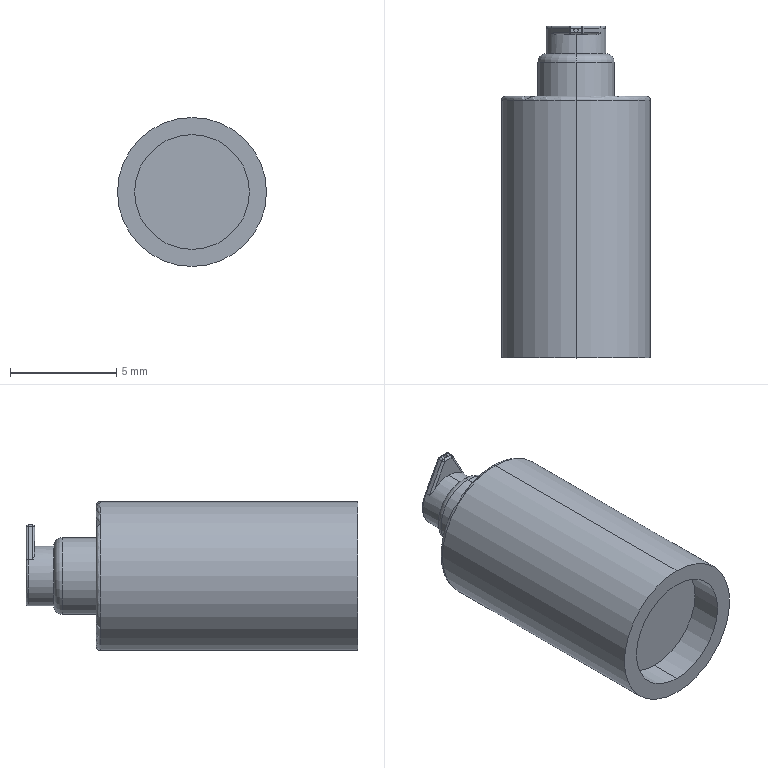Part | SolidWorks | features ICE 5, Fillet 3, Shell 2, Extrusion 1 | 1 solid | 47 faces | box 7 x 15.6 x 7 mm | volume 176.298 mm3 | cylinder 24 | plane 14 | torus 5 | sphere 4 | commonest cylinder face diameters 0.2 x10 1.8 x2 2.6 x2 2.8 x2 3.6 x2 5.4 x2
STEP:
#1=CARTESIAN_POINT('',(0.,12.1,-3.5));
#2=VERTEX_POINT('',#1);
#3=CARTESIAN_POINT('',(0.,12.1,3.5));
#4=VERTEX_POINT('',#3);
#5=CARTESIAN_POINT('',(0.,12.1,0.));
#6=DIRECTION('',(0.,-1.,0.));
#7=DIRECTION('',(0.,0.,1.));
#8=AXIS2_PLACEMENT_3D('',#5,#6,#7);
#9=CIRCLE('',#8,3.5);
#10=EDGE_CURVE('',#2,#4,#9,.T.);
#11=ORIENTED_EDGE('',*,*,#10,.F.);
#12=CARTESIAN_POINT('',(0.,12.3,-3.3));
#13=VERTEX_POINT('',#12);
#14=CARTESIAN_POINT('',(0.,12.1,-3.3));
#15=DIRECTION('',(1.,0.,0.));
#16=DIRECTION('',(0.,0.,-1.));
#17=AXIS2_PLACEMENT_3D('',#14,#15,#16);
#18=CIRCLE('',#17,0.2);
#19=EDGE_CURVE('',#2,#13,#18,.T.);
#20=ORIENTED_EDGE('',*,*,#19,.T.);
#21=CARTESIAN_POINT('',(0.,12.3,3.3));
#22=VERTEX_POINT('',#21);
#23=CARTESIAN_POINT('',(0.,12.3,0.));
#24=DIRECTION('',(0.,1.,0.));
#25=DIRECTION('',(0.,0.,1.));
#26=AXIS2_PLACEMENT_3D('',#23,#24,#25);
#27=CIRCLE('',#26,3.3);
#28=EDGE_CURVE('',#22,#13,#27,.T.);
#29=ORIENTED_EDGE('',*,*,#28,.F.);
#30=CARTESIAN_POINT('',(0.,12.1,3.3));
#31=DIRECTION('',(-1.,0.,0.));
#32=DIRECTION('',(0.,0.,1.));
#33=AXIS2_PLACEMENT_3D('',#30,#31,#32);
#34=CIRCLE('',#33,0.2);
#35=EDGE_CURVE('',#4,#22,#34,.T.);
#36=ORIENTED_EDGE('',*,*,#35,.F.);
#37=EDGE_LOOP('',(#11,#20,#29,#36));
#38=FACE_OUTER_BOUND('',#37,.T.);
#39=CARTESIAN_POINT('',(0.,12.1,0.));
#40=DIRECTION('',(0.,1.,0.));
#41=DIRECTION('',(0.,0.,1.));
#42=AXIS2_PLACEMENT_3D('',#39,#40,#41);
#43=TOROIDAL_SURFACE('',#42,3.3,0.2);
#44=ADVANCED_FACE('',(#38),#43,.T.);
#45=CARTESIAN_POINT('',(0.,13.9,-1.8));
#46=VERTEX_POINT('',#45);
#47=CARTESIAN_POINT('',(0.,13.9,1.8));
#48=VERTEX_POINT('',#47);
#49=CARTESIAN_POINT('',(0.,13.9,0.));
#50=DIRECTION('',(0.,-1.,0.));
#51=DIRECTION('',(0.,0.,1.));
#52=AXIS2_PLACEMENT_3D('',#49,#50,#51);
#53=CIRCLE('',#52,1.8);
#54=EDGE_CURVE('',#46,#48,#53,.T.);
#55=ORIENTED_EDGE('',*,*,#54,.F.);
#56=CARTESIAN_POINT('',(0.,14.3,-1.4));
#57=VERTEX_POINT('',#56);
#58=CARTESIAN_POINT('',(0.,13.9,-1.4));
#59=DIRECTION('',(1.,0.,0.));
#60=DIRECTION('',(0.,0.,-1.));
#61=AXIS2_PLACEMENT_3D('',#58,#59,#60);
#62=CIRCLE('',#61,0.4);
#63=EDGE_CURVE('',#46,#57,#62,.T.);
#64=ORIENTED_EDGE('',*,*,#63,.T.);
#65=CARTESIAN_POINT('',(0.,14.3,1.4));
#66=VERTEX_POINT('',#65);
#67=CARTESIAN_POINT('',(0.,14.3,0.));
#68=DIRECTION('',(0.,1.,0.));
#69=DIRECTION('',(0.,0.,1.));
#70=AXIS2_PLACEMENT_3D('',#67,#68,#69);
#71=CIRCLE('',#70,1.4);
#72=EDGE_CURVE('',#66,#57,#71,.T.);
#73=ORIENTED_EDGE('',*,*,#72,.F.);
#74=CARTESIAN_POINT('',(0.,13.9,1.4));
#75=DIRECTION('',(-1.,0.,0.));
#76=DIRECTION('',(0.,0.,1.));
#77=AXIS2_PLACEMENT_3D('',#74,#75,#76);
#78=CIRCLE('',#77,0.4);
#79=EDGE_CURVE('',#48,#66,#78,.T.);
#80=ORIENTED_EDGE('',*,*,#79,.F.);
#81=EDGE_LOOP('',(#55,#64,#73,#80));
#82=FACE_OUTER_BOUND('',#81,.T.);
#83=CARTESIAN_POINT('',(0.,13.9,0.));
#84=DIRECTION('',(0.,1.,0.));
#85=DIRECTION('',(0.,0.,1.));
#86=AXIS2_PLACEMENT_3D('',#83,#84,#85);
#87=TOROIDAL_SURFACE('',#86,1.4,0.4);
#88=ADVANCED_FACE('',(#82),#87,.T.);
#89=CARTESIAN_POINT('',(-0.1,15.4,2.));
#90=VERTEX_POINT('',#89);
#91=CARTESIAN_POINT('',(0.1,15.4,2.));
#92=VERTEX_POINT('',#91);
#93=CARTESIAN_POINT('',(0.,15.4,2.));
#94=DIRECTION('',(0.,0.,1.));
#95=DIRECTION('',(1.,0.,0.));
#96=AXIS2_PLACEMENT_3D('',#93,#94,#95);
#97=CIRCLE('',#96,0.1);
#98=EDGE_CURVE('',#90,#92,#97,.T.);
#99=ORIENTED_EDGE('',*,*,#98,.F.);
#100=CARTESIAN_POINT('',(-0.1,15.4,2.4));
#101=VERTEX_POINT('',#100);
#102=CARTESIAN_POINT('',(-0.1,15.4,2.));
#103=DIRECTION('',(0.,0.,1.));
#104=VECTOR('',#103,1000.);
#105=LINE('',#102,#104);
#106=EDGE_CURVE('',#90,#101,#105,.T.);
#107=ORIENTED_EDGE('',*,*,#106,.T.);
#108=CARTESIAN_POINT('',(0.,15.3,2.4));
#109=VERTEX_POINT('',#108);
#110=CARTESIAN_POINT('',(0.,15.4,2.4));
#111=DIRECTION('',(0.,0.,1.));
#112=DIRECTION('',(1.,0.,0.));
#113=AXIS2_PLACEMENT_3D('',#110,#111,#112);
#114=CIRCLE('',#113,0.1);
#115=EDGE_CURVE('',#101,#109,#114,.T.);
#116=ORIENTED_EDGE('',*,*,#115,.T.);
#117=CARTESIAN_POINT('',(0.1,15.4,2.4));
#118=VERTEX_POINT('',#117);
#119=CARTESIAN_POINT('',(0.,15.4,2.4));
#120=DIRECTION('',(0.,0.,1.));
#121=DIRECTION('',(1.,0.,0.));
#122=AXIS2_PLACEMENT_3D('',#119,#120,#121);
#123=CIRCLE('',#122,0.1);
#124=EDGE_CURVE('',#109,#118,#123,.T.);
#125=ORIENTED_EDGE('',*,*,#124,.T.);
#126=CARTESIAN_POINT('',(0.1,15.4,2.));
#127=DIRECTION('',(0.,0.,1.));
#128=VECTOR('',#127,1000.);
#129=LINE('',#126,#128);
#130=EDGE_CURVE('',#92,#118,#129,.T.);
#131=ORIENTED_EDGE('',*,*,#130,.F.);
#132=EDGE_LOOP('',(#99,#107,#116,#125,#131));
#133=FACE_OUTER_BOUND('',#132,.T.);
#134=CARTESIAN_POINT('',(0.,15.4,2.));
#135=DIRECTION('',(0.,0.,1.));
#136=DIRECTION('',(1.,0.,0.));
#137=AXIS2_PLACEMENT_3D('',#134,#135,#136);
#138=CYLINDRICAL_SURFACE('',#137,0.1);
#139=ADVANCED_FACE('',(#133),#138,.F.);
#140=CARTESIAN_POINT('',(0.,15.2,1.4));
#141=VERTEX_POINT('',#140);
#142=CARTESIAN_POINT('',(0.891,15.2,1.08));
#143=VERTEX_POINT('',#142);
#144=CARTESIAN_POINT('',(0.,15.2,0.));
#145=DIRECTION('',(0.,1.,0.));
#146=DIRECTION('',(0.,0.,1.));
#147=AXIS2_PLACEMENT_3D('',#144,#145,#146);
#148=CIRCLE('',#147,1.4);
#149=EDGE_CURVE('',#141,#143,#148,.T.);
#150=ORIENTED_EDGE('',*,*,#149,.F.);
#151=CARTESIAN_POINT('',(0.,15.6,1.4));
#152=DIRECTION('',(0.,-1.,0.));
#153=VECTOR('',#152,1000.);
#154=LINE('',#151,#153);
#155=EDGE_CURVE('',#141,#66,#154,.T.);
#156=ORIENTED_EDGE('',*,*,#155,.T.);
#157=ORIENTED_EDGE('',*,*,#72,.T.);
#158=CARTESIAN_POINT('',(0.,15.5,-1.4));
#159=VERTEX_POINT('',#158);
#160=CARTESIAN_POINT('',(0.,15.6,-1.4));
#161=DIRECTION('',(0.,-1.,0.));
#162=VECTOR('',#161,1000.);
#163=LINE('',#160,#162);
#164=EDGE_CURVE('',#159,#57,#163,.T.);
#165=ORIENTED_EDGE('',*,*,#164,.F.);
#166=CARTESIAN_POINT('',(1.171,15.5,0.7666));
#167=VERTEX_POINT('',#166);
#168=CARTESIAN_POINT('',(0.,15.5,0.));
#169=DIRECTION('',(0.,-1.,0.));
#170=DIRECTION('',(0.,0.,1.));
#171=AXIS2_PLACEMENT_3D('',#168,#169,#170);
#172=CIRCLE('',#171,1.4);
#173=EDGE_CURVE('',#159,#167,#172,.T.);
#174=ORIENTED_EDGE('',*,*,#173,.T.);
#175=CARTESIAN_POINT('',(1.171,15.3,0.7666));
#176=VERTEX_POINT('',#175);
#177=CARTESIAN_POINT('',(1.171,15.2,0.7666));
#178=DIRECTION('',(0.,1.,0.));
#179=VECTOR('',#178,1000.);
#180=LINE('',#177,#179);
#181=EDGE_CURVE('',#176,#167,#180,.T.);
#182=ORIENTED_EDGE('',*,*,#181,.F.);
#183=CARTESIAN_POINT('',(1.171,15.3,0.7666));
#184=CARTESIAN_POINT('',(1.171,15.291,0.7666));
#185=CARTESIAN_POINT('',(1.166,15.285,0.7756));
#186=CARTESIAN_POINT('',(1.156,15.277,0.7891));
#187=CARTESIAN_POINT('',(1.152,15.273,0.7961));
#188=CARTESIAN_POINT('',(1.137,15.263,0.8173));
#189=CARTESIAN_POINT('',(1.126,15.258,0.8315));
#190=CARTESIAN_POINT('',(1.095,15.242,0.8737));
#191=CARTESIAN_POINT('',(1.072,15.234,0.9012));
#192=CARTESIAN_POINT('',(1.,15.211,0.9819));
#193=CARTESIAN_POINT('',(0.9479,15.2,1.033));
#194=CARTESIAN_POINT('',(0.891,15.2,1.08));
#195=B_SPLINE_CURVE_WITH_KNOTS('',3,(#183,#184,#185,#186,#187,#188,#189,#190,#191,#192,#193,#194),.UNSPECIFIED.,.F.,.F.,(4,2,2,2,2,4),(0.,0.00002786,0.00005573,0.0001115,0.0002229,0.0004458),.UNSPECIFIED.);
#196=EDGE_CURVE('',#176,#143,#195,.T.);
#197=ORIENTED_EDGE('',*,*,#196,.T.);
#198=EDGE_LOOP('',(#150,#156,#157,#165,#174,#182,#197));
#199=FACE_OUTER_BOUND('',#198,.T.);
#200=CARTESIAN_POINT('',(0.,15.6,0.));
#201=DIRECTION('',(0.,-1.,0.));
#202=DIRECTION('',(0.,0.,-1.));
#203=AXIS2_PLACEMENT_3D('',#200,#201,#202);
#204=CYLINDRICAL_SURFACE('',#203,1.4);
#205=ADVANCED_FACE('',(#199),#204,.T.);
#206=ORIENTED_EDGE('',*,*,#54,.T.);
#207=CARTESIAN_POINT('',(0.,12.3,1.8));
#208=VERTEX_POINT('',#207);
#209=CARTESIAN_POINT('',(0.,14.3,1.8));
#210=DIRECTION('',(0.,-1.,0.));
#211=VECTOR('',#210,1000.);
#212=LINE('',#209,#211);
#213=EDGE_CURVE('',#48,#208,#212,.T.);
#214=ORIENTED_EDGE('',*,*,#213,.T.);
#215=CARTESIAN_POINT('',(0.,12.3,-1.8));
#216=VERTEX_POINT('',#215);
#217=CARTESIAN_POINT('',(0.,12.3,0.));
#218=DIRECTION('',(0.,1.,0.));
#219=DIRECTION('',(0.,0.,1.));
#220=AXIS2_PLACEMENT_3D('',#217,#218,#219);
#221=CIRCLE('',#220,1.8);
#222=EDGE_CURVE('',#208,#216,#221,.T.);
#223=ORIENTED_EDGE('',*,*,#222,.T.);
#224=CARTESIAN_POINT('',(0.,14.3,-1.8));
#225=DIRECTION('',(0.,-1.,0.));
#226=VECTOR('',#225,1000.);
#227=LINE('',#224,#226);
#228=EDGE_CURVE('',#46,#216,#227,.T.);
#229=ORIENTED_EDGE('',*,*,#228,.F.);
#230=EDGE_LOOP('',(#206,#214,#223,#229));
#231=FACE_OUTER_BOUND('',#230,.T.);
#232=CARTESIAN_POINT('',(0.,14.3,0.));
#233=DIRECTION('',(0.,-1.,0.));
#234=DIRECTION('',(0.,0.,-1.));
#235=AXIS2_PLACEMENT_3D('',#232,#233,#234);
#236=CYLINDRICAL_SURFACE('',#235,1.8);
#237=ADVANCED_FACE('',(#231),#236,.T.);
#238=CARTESIAN_POINT('',(0.,1.5,-2.7));
#239=VERTEX_POINT('',#238);
#240=CARTESIAN_POINT('',(0.,1.5,2.7));
#241=VERTEX_POINT('',#240);
#242=CARTESIAN_POINT('',(0.,1.5,0.));
#243=DIRECTION('',(0.,1.,0.));
#244=DIRECTION('',(0.,0.,1.));
#245=AXIS2_PLACEMENT_3D('',#242,#243,#244);
#246=CIRCLE('',#245,2.7);
#247=EDGE_CURVE('',#239,#241,#246,.T.);
#248=ORIENTED_EDGE('',*,*,#247,.T.);
#249=CARTESIAN_POINT('',(0.,0.,2.7));
#250=VERTEX_POINT('',#249);
#251=CARTESIAN_POINT('',(0.,2.3,2.7));
#252=DIRECTION('',(0.,-1.,0.));
#253=VECTOR('',#252,1000.);
#254=LINE('',#251,#253);
#255=EDGE_CURVE('',#241,#250,#254,.T.);
#256=ORIENTED_EDGE('',*,*,#255,.T.);
#257=CARTESIAN_POINT('',(0.,0.,-2.7));
#258=VERTEX_POINT('',#257);
#259=CARTESIAN_POINT('',(0.,0.,0.));
#260=DIRECTION('',(0.,1.,0.));
#261=DIRECTION('',(0.,0.,1.));
#262=AXIS2_PLACEMENT_3D('',#259,#260,#261);
#263=CIRCLE('',#262,2.7);
#264=EDGE_CURVE('',#258,#250,#263,.T.);
#265=ORIENTED_EDGE('',*,*,#264,.F.);
#266=CARTESIAN_POINT('',(0.,2.3,-2.7));
#267=DIRECTION('',(0.,-1.,0.));
#268=VECTOR('',#267,1000.);
#269=LINE('',#266,#268);
#270=EDGE_CURVE('',#239,#258,#269,.T.);
#271=ORIENTED_EDGE('',*,*,#270,.F.);
#272=EDGE_LOOP('',(#248,#256,#265,#271));
#273=FACE_OUTER_BOUND('',#272,.T.);
#274=CARTESIAN_POINT('',(0.,2.3,0.));
#275=DIRECTION('',(0.,-1.,0.));
#276=DIRECTION('',(0.,0.,-1.));
#277=AXIS2_PLACEMENT_3D('',#274,#275,#276);
#278=CYLINDRICAL_SURFACE('',#277,2.7);
#279=ADVANCED_FACE('',(#273),#278,.F.);
#280=ORIENTED_EDGE('',*,*,#10,.T.);
#281=CARTESIAN_POINT('',(0.,0.,3.5));
#282=VERTEX_POINT('',#281);
#283=CARTESIAN_POINT('',(0.,2.3,3.5));
#284=DIRECTION('',(0.,-1.,0.));
#285=VECTOR('',#284,1000.);
#286=LINE('',#283,#285);
#287=EDGE_CURVE('',#4,#282,#286,.T.);
#288=ORIENTED_EDGE('',*,*,#287,.T.);
#289=CARTESIAN_POINT('',(0.,0.,-3.5));
#290=VERTEX_POINT('',#289);
#291=CARTESIAN_POINT('',(0.,0.,0.));
#292=DIRECTION('',(0.,1.,0.));
#293=DIRECTION('',(0.,0.,1.));
#294=AXIS2_PLACEMENT_3D('',#291,#292,#293);
#295=CIRCLE('',#294,3.5);
#296=EDGE_CURVE('',#282,#290,#295,.T.);
#297=ORIENTED_EDGE('',*,*,#296,.T.);
#298=CARTESIAN_POINT('',(0.,2.3,-3.5));
#299=DIRECTION('',(0.,-1.,0.));
#300=VECTOR('',#299,1000.);
#301=LINE('',#298,#300);
#302=EDGE_CURVE('',#2,#290,#301,.T.);
#303=ORIENTED_EDGE('',*,*,#302,.F.);
#304=EDGE_LOOP('',(#280,#288,#297,#303));
#305=FACE_OUTER_BOUND('',#304,.T.);
#306=CARTESIAN_POINT('',(0.,2.3,0.));
#307=DIRECTION('',(0.,-1.,0.));
#308=DIRECTION('',(0.,0.,-1.));
#309=AXIS2_PLACEMENT_3D('',#306,#307,#308);
#310=CYLINDRICAL_SURFACE('',#309,3.5);
#311=ADVANCED_FACE('',(#305),#310,.T.);
#312=CARTESIAN_POINT('',(0.24,15.3,2.4));
#313=VERTEX_POINT('',#312);
#314=CARTESIAN_POINT('',(0.24,15.5,2.4));
#315=VERTEX_POINT('',#314);
#316=CARTESIAN_POINT('',(0.24,15.2,2.4));
#317=DIRECTION('',(0.,1.,0.));
#318=VECTOR('',#317,1000.);
#319=LINE('',#316,#318);
#320=EDGE_CURVE('',#313,#315,#319,.T.);
#321=ORIENTED_EDGE('',*,*,#320,.T.);
#322=CARTESIAN_POINT('',(0.,15.5,2.4));
#323=VERTEX_POINT('',#322);
#324=CARTESIAN_POINT('',(-0.3,15.5,2.4));
#325=DIRECTION('',(-1.,0.,0.));
#326=VECTOR('',#325,1000.);
#327=LINE('',#324,#326);
#328=EDGE_CURVE('',#315,#323,#327,.T.);
#329=ORIENTED_EDGE('',*,*,#328,.T.);
#330=CARTESIAN_POINT('',(0.,15.4,2.4));
#331=DIRECTION('',(0.,0.,1.));
#332=DIRECTION('',(1.,0.,0.));
#333=AXIS2_PLACEMENT_3D('',#330,#331,#332);
#334=CIRCLE('',#333,0.1);
#335=EDGE_CURVE('',#118,#323,#334,.T.);
#336=ORIENTED_EDGE('',*,*,#335,.F.);
#337=ORIENTED_EDGE('',*,*,#124,.F.);
#338=CARTESIAN_POINT('',(0.3,15.3,2.4));
#339=DIRECTION('',(1.,0.,0.));
#340=VECTOR('',#339,1000.);
#341=LINE('',#338,#340);
#342=EDGE_CURVE('',#109,#313,#341,.T.);
#343=ORIENTED_EDGE('',*,*,#342,.T.);
#344=EDGE_LOOP('',(#321,#329,#336,#337,#343));
#345=FACE_OUTER_BOUND('',#344,.T.);
#346=CARTESIAN_POINT('',(-0.3,15.2,2.4));
#347=DIRECTION('',(0.,0.,1.));
#348=DIRECTION('',(1.,0.,0.));
#349=AXIS2_PLACEMENT_3D('',#346,#347,#348);
#350=PLANE('',#349);
#351=ADVANCED_FACE('',(#345),#350,.T.);
#352=ORIENTED_EDGE('',*,*,#287,.F.);
#353=CARTESIAN_POINT('',(0.,12.1,0.));
#354=DIRECTION('',(0.,-1.,0.));
#355=DIRECTION('',(0.,0.,1.));
#356=AXIS2_PLACEMENT_3D('',#353,#354,#355);
#357=CIRCLE('',#356,3.5);
#358=EDGE_CURVE('',#4,#2,#357,.T.);
#359=ORIENTED_EDGE('',*,*,#358,.T.);
#360=ORIENTED_EDGE('',*,*,#302,.T.);
#361=CARTESIAN_POINT('',(0.,0.,0.));
#362=DIRECTION('',(0.,1.,0.));
#363=DIRECTION('',(0.,0.,1.));
#364=AXIS2_PLACEMENT_3D('',#361,#362,#363);
#365=CIRCLE('',#364,3.5);
#366=EDGE_CURVE('',#290,#282,#365,.T.);
#367=ORIENTED_EDGE('',*,*,#366,.T.);
#368=EDGE_LOOP('',(#352,#359,#360,#367));
#369=FACE_OUTER_BOUND('',#368,.T.);
#370=CARTESIAN_POINT('',(0.,2.3,0.));
#371=DIRECTION('',(0.,-1.,0.));
#372=DIRECTION('',(0.,0.,-1.));
#373=AXIS2_PLACEMENT_3D('',#370,#371,#372);
#374=CYLINDRICAL_SURFACE('',#373,3.5);
#375=ADVANCED_FACE('',(#369),#374,.T.);
#376=ORIENTED_EDGE('',*,*,#264,.T.);
#377=CARTESIAN_POINT('',(0.,0.,0.));
#378=DIRECTION('',(0.,1.,0.));
#379=DIRECTION('',(0.,0.,1.));
#380=AXIS2_PLACEMENT_3D('',#377,#378,#379);
#381=CIRCLE('',#380,2.7);
#382=EDGE_CURVE('',#250,#258,#381,.T.);
#383=ORIENTED_EDGE('',*,*,#382,.T.);
#384=EDGE_LOOP('',(#376,#383));
#385=FACE_BOUND('',#384,.T.);
#386=ORIENTED_EDGE('',*,*,#366,.F.);
#387=ORIENTED_EDGE('',*,*,#296,.F.);
#388=EDGE_LOOP('',(#386,#387));
#389=FACE_OUTER_BOUND('',#388,.T.);
#390=CARTESIAN_POINT('',(0.,0.,0.));
#391=DIRECTION('',(0.,1.,0.));
#392=DIRECTION('',(0.,0.,1.));
#393=AXIS2_PLACEMENT_3D('',#390,#391,#392);
#394=PLANE('',#393);
#395=ADVANCED_FACE('',(#385,#389),#394,.F.);
#396=ORIENTED_EDGE('',*,*,#255,.F.);
#397=CARTESIAN_POINT('',(0.,1.5,0.));
#398=DIRECTION('',(0.,1.,0.));
#399=DIRECTION('',(0.,0.,1.));
#400=AXIS2_PLACEMENT_3D('',#397,#398,#399);
#401=CIRCLE('',#400,2.7);
#402=EDGE_CURVE('',#241,#239,#401,.T.);
#403=ORIENTED_EDGE('',*,*,#402,.T.);
#404=ORIENTED_EDGE('',*,*,#270,.T.);
#405=ORIENTED_EDGE('',*,*,#382,.F.);
#406=EDGE_LOOP('',(#396,#403,#404,#405));
#407=FACE_OUTER_BOUND('',#406,.T.);
#408=CARTESIAN_POINT('',(0.,2.3,0.));
#409=DIRECTION('',(0.,-1.,0.));
#410=DIRECTION('',(0.,0.,-1.));
#411=AXIS2_PLACEMENT_3D('',#408,#409,#410);
#412=CYLINDRICAL_SURFACE('',#411,2.7);
#413=ADVANCED_FACE('',(#407),#412,.F.);
#414=ORIENTED_EDGE('',*,*,#247,.F.);
#415=ORIENTED_EDGE('',*,*,#402,.F.);
#416=EDGE_LOOP('',(#414,#415));
#417=FACE_OUTER_BOUND('',#416,.T.);
#418=CARTESIAN_POINT('',(0.,1.5,0.));
#419=DIRECTION('',(0.,1.,0.));
#420=DIRECTION('',(0.,0.,1.));
#421=AXIS2_PLACEMENT_3D('',#418,#419,#420);
#422=PLANE('',#421);
#423=ADVANCED_FACE('',(#417),#422,.F.);
#424=ORIENTED_EDGE('',*,*,#28,.T.);
#425=CARTESIAN_POINT('',(0.,12.3,0.));
#426=DIRECTION('',(0.,1.,0.));
#427=DIRECTION('',(0.,0.,1.));
#428=AXIS2_PLACEMENT_3D('',#425,#426,#427);
#429=CIRCLE('',#428,3.3);
#430=EDGE_CURVE('',#13,#22,#429,.T.);
#431=ORIENTED_EDGE('',*,*,#430,.T.);
#432=EDGE_LOOP('',(#424,#431));
#433=FACE_OUTER_BOUND('',#432,.T.);
#434=CARTESIAN_POINT('',(0.,12.3,0.));
#435=DIRECTION('',(0.,1.,0.));
#436=DIRECTION('',(0.,0.,1.));
#437=AXIS2_PLACEMENT_3D('',#434,#435,#436);
#438=CIRCLE('',#437,1.8);
#439=EDGE_CURVE('',#216,#208,#438,.T.);
#440=ORIENTED_EDGE('',*,*,#439,.F.);
#441=ORIENTED_EDGE('',*,*,#222,.F.);
#442=EDGE_LOOP('',(#440,#441));
#443=FACE_BOUND('',#442,.T.);
#444=CARTESIAN_POINT('',(0.,12.3,0.));
#445=DIRECTION('',(0.,1.,0.));
#446=DIRECTION('',(0.,0.,1.));
#447=AXIS2_PLACEMENT_3D('',#444,#445,#446);
#448=PLANE('',#447);
#449=ADVANCED_FACE('',(#433,#443),#448,.T.);
#450=ORIENTED_EDGE('',*,*,#213,.F.);
#451=CARTESIAN_POINT('',(0.,13.9,0.));
#452=DIRECTION('',(0.,-1.,0.));
#453=DIRECTION('',(0.,0.,1.));
#454=AXIS2_PLACEMENT_3D('',#451,#452,#453);
#455=CIRCLE('',#454,1.8);
#456=EDGE_CURVE('',#48,#46,#455,.T.);
#457=ORIENTED_EDGE('',*,*,#456,.T.);
#458=ORIENTED_EDGE('',*,*,#228,.T.);
#459=ORIENTED_EDGE('',*,*,#439,.T.);
#460=EDGE_LOOP('',(#450,#457,#458,#459));
#461=FACE_OUTER_BOUND('',#460,.T.);
#462=CARTESIAN_POINT('',(0.,14.3,0.));
#463=DIRECTION('',(0.,-1.,0.));
#464=DIRECTION('',(0.,0.,-1.));
#465=AXIS2_PLACEMENT_3D('',#462,#463,#464);
#466=CYLINDRICAL_SURFACE('',#465,1.8);
#467=ADVANCED_FACE('',(#461),#466,.T.);
#468=ORIENTED_EDGE('',*,*,#155,.F.);
#469=CARTESIAN_POINT('',(-0.891,15.2,1.08));
#470=VERTEX_POINT('',#469);
#471=CARTESIAN_POINT('',(0.,15.2,0.));
#472=DIRECTION('',(0.,1.,0.));
#473=DIRECTION('',(0.,0.,1.));
#474=AXIS2_PLACEMENT_3D('',#471,#472,#473);
#475=CIRCLE('',#474,1.4);
#476=EDGE_CURVE('',#470,#141,#475,.T.);
#477=ORIENTED_EDGE('',*,*,#476,.F.);
#478=CARTESIAN_POINT('',(-1.171,15.3,0.7666));
#479=VERTEX_POINT('',#478);
#480=CARTESIAN_POINT('',(-0.891,15.2,1.08));
#481=CARTESIAN_POINT('',(-0.948,15.2,1.033));
#482=CARTESIAN_POINT('',(-1.,15.211,0.9823));
#483=CARTESIAN_POINT('',(-1.072,15.234,0.9013));
#484=CARTESIAN_POINT('',(-1.095,15.242,0.8736));
#485=CARTESIAN_POINT('',(-1.127,15.258,0.8313));
#486=CARTESIAN_POINT('',(-1.137,15.263,0.8171));
#487=CARTESIAN_POINT('',(-1.152,15.273,0.796));
#488=CARTESIAN_POINT('',(-1.157,15.277,0.7889));
#489=CARTESIAN_POINT('',(-1.166,15.285,0.7755));
#490=CARTESIAN_POINT('',(-1.171,15.291,0.7666));
#491=CARTESIAN_POINT('',(-1.171,15.3,0.7666));
#492=B_SPLINE_CURVE_WITH_KNOTS('',3,(#480,#481,#482,#483,#484,#485,#486,#487,#488,#489,#490,#491),.UNSPECIFIED.,.F.,.F.,(4,2,2,2,2,4),(0.,0.0002198,0.0003297,0.0003846,0.0004121,0.0004395),.UNSPECIFIED.);
#493=EDGE_CURVE('',#470,#479,#492,.T.);
#494=ORIENTED_EDGE('',*,*,#493,.T.);
#495=CARTESIAN_POINT('',(-1.171,15.5,0.7666));
#496=VERTEX_POINT('',#495);
#497=CARTESIAN_POINT('',(-1.171,15.2,0.7666));
#498=DIRECTION('',(0.,1.,0.));
#499=VECTOR('',#498,1000.);
#500=LINE('',#497,#499);
#501=EDGE_CURVE('',#479,#496,#500,.T.);
#502=ORIENTED_EDGE('',*,*,#501,.T.);
#503=CARTESIAN_POINT('',(0.,15.5,0.));
#504=DIRECTION('',(0.,-1.,0.));
#505=DIRECTION('',(0.,0.,1.));
#506=AXIS2_PLACEMENT_3D('',#503,#504,#505);
#507=CIRCLE('',#506,1.4);
#508=EDGE_CURVE('',#496,#159,#507,.T.);
#509=ORIENTED_EDGE('',*,*,#508,.T.);
#510=ORIENTED_EDGE('',*,*,#164,.T.);
#511=CARTESIAN_POINT('',(0.,14.3,0.));
#512=DIRECTION('',(0.,1.,0.));
#513=DIRECTION('',(0.,0.,1.));
#514=AXIS2_PLACEMENT_3D('',#511,#512,#513);
#515=CIRCLE('',#514,1.4);
#516=EDGE_CURVE('',#57,#66,#515,.T.);
#517=ORIENTED_EDGE('',*,*,#516,.T.);
#518=EDGE_LOOP('',(#468,#477,#494,#502,#509,#510,#517));
#519=FACE_OUTER_BOUND('',#518,.T.);
#520=CARTESIAN_POINT('',(0.,15.6,0.));
#521=DIRECTION('',(0.,-1.,0.));
#522=DIRECTION('',(0.,0.,-1.));
#523=AXIS2_PLACEMENT_3D('',#520,#521,#522);
#524=CYLINDRICAL_SURFACE('',#523,1.4);
#525=ADVANCED_FACE('',(#519),#524,.T.);
#526=CARTESIAN_POINT('',(-0.24,15.6,2.3));
#527=VERTEX_POINT('',#526);
#528=CARTESIAN_POINT('',(0.24,15.6,2.3));
#529=VERTEX_POINT('',#528);
#530=CARTESIAN_POINT('',(0.,15.6,2.3));
#531=DIRECTION('',(1.,0.,0.));
#532=VECTOR('',#531,1000.);
#533=LINE('',#530,#532);
#534=EDGE_CURVE('',#527,#529,#533,.T.);
#535=ORIENTED_EDGE('',*,*,#534,.T.);
#536=CARTESIAN_POINT('',(1.085,15.6,0.7155));
#537=VERTEX_POINT('',#536);
#538=CARTESIAN_POINT('',(1.142,15.6,0.6093));
#539=DIRECTION('',(0.4707,0.,-0.8823));
#540=VECTOR('',#539,1000.);
#541=LINE('',#538,#540);
#542=EDGE_CURVE('',#529,#537,#541,.T.);
#543=ORIENTED_EDGE('',*,*,#542,.T.);
#544=CARTESIAN_POINT('',(-1.085,15.6,0.7155));
#545=VERTEX_POINT('',#544);
#546=CARTESIAN_POINT('',(0.,15.6,0.));
#547=DIRECTION('',(0.,1.,0.));
#548=DIRECTION('',(0.,0.,1.));
#549=AXIS2_PLACEMENT_3D('',#546,#547,#548);
#550=CIRCLE('',#549,1.3);
#551=EDGE_CURVE('',#537,#545,#550,.T.);
#552=ORIENTED_EDGE('',*,*,#551,.T.);
#553=CARTESIAN_POINT('',(-1.142,15.6,0.6093));
#554=DIRECTION('',(0.4707,0.,0.8823));
#555=VECTOR('',#554,1000.);
#556=LINE('',#553,#555);
#557=EDGE_CURVE('',#545,#527,#556,.T.);
#558=ORIENTED_EDGE('',*,*,#557,.T.);
#559=EDGE_LOOP('',(#535,#543,#552,#558));
#560=FACE_OUTER_BOUND('',#559,.T.);
#561=CARTESIAN_POINT('',(0.,15.6,0.));
#562=DIRECTION('',(0.,1.,0.));
#563=DIRECTION('',(0.,0.,1.));
#564=AXIS2_PLACEMENT_3D('',#561,#562,#563);
#565=PLANE('',#564);
#566=ADVANCED_FACE('',(#560),#565,.T.);
#567=ORIENTED_EDGE('',*,*,#181,.T.);
#568=CARTESIAN_POINT('',(0.3282,15.5,2.347));
#569=VERTEX_POINT('',#568);
#570=CARTESIAN_POINT('',(1.171,15.5,0.7666));
#571=DIRECTION('',(-0.4707,0.,0.8823));
#572=VECTOR('',#571,1000.);
#573=LINE('',#570,#572);
#574=EDGE_CURVE('',#167,#569,#573,.T.);
#575=ORIENTED_EDGE('',*,*,#574,.T.);
#576=CARTESIAN_POINT('',(0.3282,15.3,2.347));
#577=VERTEX_POINT('',#576);
#578=CARTESIAN_POINT('',(0.3282,15.2,2.347));
#579=DIRECTION('',(0.,-1.,0.));
#580=VECTOR('',#579,1000.);
#581=LINE('',#578,#580);
#582=EDGE_CURVE('',#569,#577,#581,.T.);
#583=ORIENTED_EDGE('',*,*,#582,.T.);
#584=CARTESIAN_POINT('',(1.171,15.3,0.7666));
#585=DIRECTION('',(0.4707,0.,-0.8823));
#586=VECTOR('',#585,1000.);
#587=LINE('',#584,#586);
#588=EDGE_CURVE('',#577,#176,#587,.T.);
#589=ORIENTED_EDGE('',*,*,#588,.T.);
#590=EDGE_LOOP('',(#567,#575,#583,#589));
#591=FACE_OUTER_BOUND('',#590,.T.);
#592=CARTESIAN_POINT('',(1.171,15.2,0.7666));
#593=DIRECTION('',(0.8823,0.,0.4707));
#594=DIRECTION('',(0.4707,0.,-0.8823));
#595=AXIS2_PLACEMENT_3D('',#592,#593,#594);
#596=PLANE('',#595);
#597=ADVANCED_FACE('',(#591),#596,.T.);
#598=CARTESIAN_POINT('',(0.,15.4,2.4));
#599=DIRECTION('',(0.,0.,1.));
#600=DIRECTION('',(1.,0.,0.));
#601=AXIS2_PLACEMENT_3D('',#598,#599,#600);
#602=CIRCLE('',#601,0.1);
#603=EDGE_CURVE('',#323,#101,#602,.T.);
#604=ORIENTED_EDGE('',*,*,#603,.F.);
#605=CARTESIAN_POINT('',(-0.24,15.5,2.4));
#606=VERTEX_POINT('',#605);
#607=CARTESIAN_POINT('',(-0.3,15.5,2.4));
#608=DIRECTION('',(-1.,0.,0.));
#609=VECTOR('',#608,1000.);
#610=LINE('',#607,#609);
#611=EDGE_CURVE('',#323,#606,#610,.T.);
#612=ORIENTED_EDGE('',*,*,#611,.T.);
#613=CARTESIAN_POINT('',(-0.24,15.3,2.4));
#614=VERTEX_POINT('',#613);
#615=CARTESIAN_POINT('',(-0.24,15.2,2.4));
#616=DIRECTION('',(0.,-1.,0.));
#617=VECTOR('',#616,1000.);
#618=LINE('',#615,#617);
#619=EDGE_CURVE('',#606,#614,#618,.T.);
#620=ORIENTED_EDGE('',*,*,#619,.T.);
#621=CARTESIAN_POINT('',(0.3,15.3,2.4));
#622=DIRECTION('',(1.,0.,0.));
#623=VECTOR('',#622,1000.);
#624=LINE('',#621,#623);
#625=EDGE_CURVE('',#614,#109,#624,.T.);
#626=ORIENTED_EDGE('',*,*,#625,.T.);
#627=ORIENTED_EDGE('',*,*,#115,.F.);
#628=EDGE_LOOP('',(#604,#612,#620,#626,#627));
#629=FACE_OUTER_BOUND('',#628,.T.);
#630=CARTESIAN_POINT('',(-0.3,15.2,2.4));
#631=DIRECTION('',(0.,0.,1.));
#632=DIRECTION('',(1.,0.,0.));
#633=AXIS2_PLACEMENT_3D('',#630,#631,#632);
#634=PLANE('',#633);
#635=ADVANCED_FACE('',(#629),#634,.T.);
#636=CARTESIAN_POINT('',(-0.3282,15.3,2.347));
#637=VERTEX_POINT('',#636);
#638=CARTESIAN_POINT('',(-0.3282,15.5,2.347));
#639=VERTEX_POINT('',#638);
#640=CARTESIAN_POINT('',(-0.3282,15.2,2.347));
#641=DIRECTION('',(0.,1.,0.));
#642=VECTOR('',#641,1000.);
#643=LINE('',#640,#642);
#644=EDGE_CURVE('',#637,#639,#643,.T.);
#645=ORIENTED_EDGE('',*,*,#644,.T.);
#646=CARTESIAN_POINT('',(-0.3,15.5,2.4));
#647=DIRECTION('',(-0.4707,0.,-0.8823));
#648=VECTOR('',#647,1000.);
#649=LINE('',#646,#648);
#650=EDGE_CURVE('',#639,#496,#649,.T.);
#651=ORIENTED_EDGE('',*,*,#650,.T.);
#652=ORIENTED_EDGE('',*,*,#501,.F.);
#653=CARTESIAN_POINT('',(-0.3,15.3,2.4));
#654=DIRECTION('',(0.4707,0.,0.8823));
#655=VECTOR('',#654,1000.);
#656=LINE('',#653,#655);
#657=EDGE_CURVE('',#479,#637,#656,.T.);
#658=ORIENTED_EDGE('',*,*,#657,.T.);
#659=EDGE_LOOP('',(#645,#651,#652,#658));
#660=FACE_OUTER_BOUND('',#659,.T.);
#661=CARTESIAN_POINT('',(-0.3,15.2,2.4));
#662=DIRECTION('',(-0.8823,0.,0.4707));
#663=DIRECTION('',(0.4707,0.,0.8823));
#664=AXIS2_PLACEMENT_3D('',#661,#662,#663);
#665=PLANE('',#664);
#666=ADVANCED_FACE('',(#660),#665,.T.);
#667=CARTESIAN_POINT('',(0.24,15.2,2.3));
#668=VERTEX_POINT('',#667);
#669=CARTESIAN_POINT('',(-0.24,15.2,2.3));
#670=VERTEX_POINT('',#669);
#671=CARTESIAN_POINT('',(-0.3,15.2,2.3));
#672=DIRECTION('',(-1.,0.,0.));
#673=VECTOR('',#672,1000.);
#674=LINE('',#671,#673);
#675=EDGE_CURVE('',#668,#670,#674,.T.);
#676=ORIENTED_EDGE('',*,*,#675,.T.);
#677=CARTESIAN_POINT('',(-1.083,15.2,0.7195));
#678=DIRECTION('',(-0.4707,0.,-0.8823));
#679=VECTOR('',#678,1000.);
#680=LINE('',#677,#679);
#681=EDGE_CURVE('',#670,#470,#680,.T.);
#682=ORIENTED_EDGE('',*,*,#681,.T.);
#683=ORIENTED_EDGE('',*,*,#476,.T.);
#684=ORIENTED_EDGE('',*,*,#149,.T.);
#685=CARTESIAN_POINT('',(0.2118,15.2,2.353));
#686=DIRECTION('',(-0.4707,0.,0.8823));
#687=VECTOR('',#686,1000.);
#688=LINE('',#685,#687);
#689=EDGE_CURVE('',#143,#668,#688,.T.);
#690=ORIENTED_EDGE('',*,*,#689,.T.);
#691=EDGE_LOOP('',(#676,#682,#683,#684,#690));
#692=FACE_OUTER_BOUND('',#691,.T.);
#693=CARTESIAN_POINT('',(0.,15.2,0.));
#694=DIRECTION('',(0.,1.,0.));
#695=DIRECTION('',(0.,0.,1.));
#696=AXIS2_PLACEMENT_3D('',#693,#694,#695);
#697=PLANE('',#696);
#698=ADVANCED_FACE('',(#692),#697,.F.);
#699=ORIENTED_EDGE('',*,*,#106,.F.);
#700=CARTESIAN_POINT('',(0.,15.4,2.));
#701=DIRECTION('',(0.,0.,1.));
#702=DIRECTION('',(1.,0.,0.));
#703=AXIS2_PLACEMENT_3D('',#700,#701,#702);
#704=CIRCLE('',#703,0.1);
#705=EDGE_CURVE('',#92,#90,#704,.T.);
#706=ORIENTED_EDGE('',*,*,#705,.F.);
#707=ORIENTED_EDGE('',*,*,#130,.T.);
#708=ORIENTED_EDGE('',*,*,#335,.T.);
#709=ORIENTED_EDGE('',*,*,#603,.T.);
#710=EDGE_LOOP('',(#699,#706,#707,#708,#709));
#711=FACE_OUTER_BOUND('',#710,.T.);
#712=CARTESIAN_POINT('',(0.,15.4,2.));
#713=DIRECTION('',(0.,0.,1.));
#714=DIRECTION('',(1.,0.,0.));
#715=AXIS2_PLACEMENT_3D('',#712,#713,#714);
#716=CYLINDRICAL_SURFACE('',#715,0.1);
#717=ADVANCED_FACE('',(#711),#716,.F.);
#718=ORIENTED_EDGE('',*,*,#705,.T.);
#719=ORIENTED_EDGE('',*,*,#98,.T.);
#720=EDGE_LOOP('',(#718,#719));
#721=FACE_OUTER_BOUND('',#720,.T.);
#722=CARTESIAN_POINT('',(0.,15.4,2.));
#723=DIRECTION('',(0.,0.,1.));
#724=DIRECTION('',(1.,0.,0.));
#725=AXIS2_PLACEMENT_3D('',#722,#723,#724);
#726=PLANE('',#725);
#727=ADVANCED_FACE('',(#721),#726,.T.);
#728=ORIENTED_EDGE('',*,*,#63,.F.);
#729=ORIENTED_EDGE('',*,*,#456,.F.);
#730=ORIENTED_EDGE('',*,*,#79,.T.);
#731=ORIENTED_EDGE('',*,*,#516,.F.);
#732=EDGE_LOOP('',(#728,#729,#730,#731));
#733=FACE_OUTER_BOUND('',#732,.T.);
#734=CARTESIAN_POINT('',(0.,13.9,0.));
#735=DIRECTION('',(0.,1.,0.));
#736=DIRECTION('',(0.,0.,1.));
#737=AXIS2_PLACEMENT_3D('',#734,#735,#736);
#738=TOROIDAL_SURFACE('',#737,1.4,0.4);
#739=ADVANCED_FACE('',(#733),#738,.T.);
#740=ORIENTED_EDGE('',*,*,#19,.F.);
#741=ORIENTED_EDGE('',*,*,#358,.F.);
#742=ORIENTED_EDGE('',*,*,#35,.T.);
#743=ORIENTED_EDGE('',*,*,#430,.F.);
#744=EDGE_LOOP('',(#740,#741,#742,#743));
#745=FACE_OUTER_BOUND('',#744,.T.);
#746=CARTESIAN_POINT('',(0.,12.1,0.));
#747=DIRECTION('',(0.,1.,0.));
#748=DIRECTION('',(0.,0.,1.));
#749=AXIS2_PLACEMENT_3D('',#746,#747,#748);
#750=TOROIDAL_SURFACE('',#749,3.3,0.2);
#751=ADVANCED_FACE('',(#745),#750,.T.);
#752=CARTESIAN_POINT('',(-0.24,15.3,2.3));
#753=DIRECTION('',(0.4707,0.,0.8823));
#754=DIRECTION('',(0.8823,0.,-0.4707));
#755=AXIS2_PLACEMENT_3D('',#752,#753,#754);
#756=CIRCLE('',#755,0.1);
#757=EDGE_CURVE('',#637,#670,#756,.T.);
#758=ORIENTED_EDGE('',*,*,#757,.F.);
#759=ORIENTED_EDGE('',*,*,#657,.F.);
#760=ORIENTED_EDGE('',*,*,#493,.F.);
#761=ORIENTED_EDGE('',*,*,#681,.F.);
#762=EDGE_LOOP('',(#758,#759,#760,#761));
#763=FACE_OUTER_BOUND('',#762,.T.);
#764=CARTESIAN_POINT('',(-0.2118,15.3,2.353));
#765=DIRECTION('',(-0.4707,0.,-0.8823));
#766=DIRECTION('',(-0.8823,0.,0.4707));
#767=AXIS2_PLACEMENT_3D('',#764,#765,#766);
#768=CYLINDRICAL_SURFACE('',#767,0.1);
#769=ADVANCED_FACE('',(#763),#768,.T.);
#770=CARTESIAN_POINT('',(-0.24,15.3,2.3));
#771=DIRECTION('',(0.,1.,0.));
#772=DIRECTION('',(0.,0.,-1.));
#773=AXIS2_PLACEMENT_3D('',#770,#771,#772);
#774=CIRCLE('',#773,0.1);
#775=EDGE_CURVE('',#637,#614,#774,.T.);
#776=ORIENTED_EDGE('',*,*,#775,.F.);
#777=ORIENTED_EDGE('',*,*,#757,.T.);
#778=CARTESIAN_POINT('',(-0.24,15.3,2.3));
#779=DIRECTION('',(1.,0.,0.));
#780=DIRECTION('',(0.,0.,1.));
#781=AXIS2_PLACEMENT_3D('',#778,#779,#780);
#782=CIRCLE('',#781,0.1);
#783=EDGE_CURVE('',#614,#670,#782,.T.);
#784=ORIENTED_EDGE('',*,*,#783,.F.);
#785=EDGE_LOOP('',(#776,#777,#784));
#786=FACE_OUTER_BOUND('',#785,.T.);
#787=CARTESIAN_POINT('',(-0.24,15.3,2.3));
#788=DIRECTION('',(0.,0.,1.));
#789=DIRECTION('',(1.,0.,0.));
#790=AXIS2_PLACEMENT_3D('',#787,#788,#789);
#791=SPHERICAL_SURFACE('',#790,0.1);
#792=ADVANCED_FACE('',(#786),#791,.T.);
#793=ORIENTED_EDGE('',*,*,#196,.F.);
#794=ORIENTED_EDGE('',*,*,#588,.F.);
#795=CARTESIAN_POINT('',(0.24,15.3,2.3));
#796=DIRECTION('',(-0.4707,0.,0.8823));
#797=DIRECTION('',(0.8823,0.,0.4707));
#798=AXIS2_PLACEMENT_3D('',#795,#796,#797);
#799=CIRCLE('',#798,0.1);
#800=EDGE_CURVE('',#668,#577,#799,.T.);
#801=ORIENTED_EDGE('',*,*,#800,.F.);
#802=ORIENTED_EDGE('',*,*,#689,.F.);
#803=EDGE_LOOP('',(#793,#794,#801,#802));
#804=FACE_OUTER_BOUND('',#803,.T.);
#805=CARTESIAN_POINT('',(1.083,15.3,0.7195));
#806=DIRECTION('',(-0.4707,0.,0.8823));
#807=DIRECTION('',(0.8823,0.,0.4707));
#808=AXIS2_PLACEMENT_3D('',#805,#806,#807);
#809=CYLINDRICAL_SURFACE('',#808,0.1);
#810=ADVANCED_FACE('',(#804),#809,.T.);
#811=ORIENTED_EDGE('',*,*,#783,.T.);
#812=ORIENTED_EDGE('',*,*,#675,.F.);
#813=CARTESIAN_POINT('',(0.24,15.3,2.3));
#814=DIRECTION('',(1.,0.,0.));
#815=DIRECTION('',(0.,1.,0.));
#816=AXIS2_PLACEMENT_3D('',#813,#814,#815);
#817=CIRCLE('',#816,0.1);
#818=EDGE_CURVE('',#313,#668,#817,.T.);
#819=ORIENTED_EDGE('',*,*,#818,.F.);
#820=ORIENTED_EDGE('',*,*,#342,.F.);
#821=ORIENTED_EDGE('',*,*,#625,.F.);
#822=EDGE_LOOP('',(#811,#812,#819,#820,#821));
#823=FACE_OUTER_BOUND('',#822,.T.);
#824=CARTESIAN_POINT('',(-0.3,15.3,2.3));
#825=DIRECTION('',(-1.,0.,0.));
#826=DIRECTION('',(0.,0.,1.));
#827=AXIS2_PLACEMENT_3D('',#824,#825,#826);
#828=CYLINDRICAL_SURFACE('',#827,0.1);
#829=ADVANCED_FACE('',(#823),#828,.T.);
#830=ORIENTED_EDGE('',*,*,#775,.T.);
#831=ORIENTED_EDGE('',*,*,#619,.F.);
#832=CARTESIAN_POINT('',(-0.24,15.5,2.3));
#833=DIRECTION('',(0.,1.,0.));
#834=DIRECTION('',(0.,0.,1.));
#835=AXIS2_PLACEMENT_3D('',#832,#833,#834);
#836=CIRCLE('',#835,0.1);
#837=EDGE_CURVE('',#639,#606,#836,.T.);
#838=ORIENTED_EDGE('',*,*,#837,.F.);
#839=ORIENTED_EDGE('',*,*,#644,.F.);
#840=EDGE_LOOP('',(#830,#831,#838,#839));
#841=FACE_OUTER_BOUND('',#840,.T.);
#842=CARTESIAN_POINT('',(-0.24,15.2,2.3));
#843=DIRECTION('',(0.,1.,0.));
#844=DIRECTION('',(0.,0.,1.));
#845=AXIS2_PLACEMENT_3D('',#842,#843,#844);
#846=CYLINDRICAL_SURFACE('',#845,0.1);
#847=ADVANCED_FACE('',(#841),#846,.T.);
#848=ORIENTED_EDGE('',*,*,#818,.T.);
#849=ORIENTED_EDGE('',*,*,#800,.T.);
#850=CARTESIAN_POINT('',(0.24,15.3,2.3));
#851=DIRECTION('',(0.,1.,0.));
#852=DIRECTION('',(0.,0.,-1.));
#853=AXIS2_PLACEMENT_3D('',#850,#851,#852);
#854=CIRCLE('',#853,0.1);
#855=EDGE_CURVE('',#313,#577,#854,.T.);
#856=ORIENTED_EDGE('',*,*,#855,.F.);
#857=EDGE_LOOP('',(#848,#849,#856));
#858=FACE_OUTER_BOUND('',#857,.T.);
#859=CARTESIAN_POINT('',(0.24,15.3,2.3));
#860=DIRECTION('',(0.,0.,1.));
#861=DIRECTION('',(1.,0.,0.));
#862=AXIS2_PLACEMENT_3D('',#859,#860,#861);
#863=SPHERICAL_SURFACE('',#862,0.1);
#864=ADVANCED_FACE('',(#858),#863,.T.);
#865=CARTESIAN_POINT('',(-0.24,15.5,2.3));
#866=DIRECTION('',(-0.4707,0.,-0.8823));
#867=DIRECTION('',(0.8823,0.,-0.4707));
#868=AXIS2_PLACEMENT_3D('',#865,#866,#867);
#869=CIRCLE('',#868,0.1);
#870=EDGE_CURVE('',#639,#527,#869,.T.);
#871=ORIENTED_EDGE('',*,*,#870,.F.);
#872=ORIENTED_EDGE('',*,*,#837,.T.);
#873=CARTESIAN_POINT('',(-0.24,15.5,2.3));
#874=DIRECTION('',(1.,0.,0.));
#875=DIRECTION('',(0.,-1.,0.));
#876=AXIS2_PLACEMENT_3D('',#873,#874,#875);
#877=CIRCLE('',#876,0.1);
#878=EDGE_CURVE('',#527,#606,#877,.T.);
#879=ORIENTED_EDGE('',*,*,#878,.F.);
#880=EDGE_LOOP('',(#871,#872,#879));
#881=FACE_OUTER_BOUND('',#880,.T.);
#882=CARTESIAN_POINT('',(-0.24,15.5,2.3));
#883=DIRECTION('',(0.,0.,1.));
#884=DIRECTION('',(-1.,0.,0.));
#885=AXIS2_PLACEMENT_3D('',#882,#883,#884);
#886=SPHERICAL_SURFACE('',#885,0.1);
#887=ADVANCED_FACE('',(#881),#886,.T.);
#888=ORIENTED_EDGE('',*,*,#855,.T.);
#889=ORIENTED_EDGE('',*,*,#582,.F.);
#890=CARTESIAN_POINT('',(0.24,15.5,2.3));
#891=DIRECTION('',(0.,1.,0.));
#892=DIRECTION('',(0.,0.,1.));
#893=AXIS2_PLACEMENT_3D('',#890,#891,#892);
#894=CIRCLE('',#893,0.1);
#895=EDGE_CURVE('',#315,#569,#894,.T.);
#896=ORIENTED_EDGE('',*,*,#895,.F.);
#897=ORIENTED_EDGE('',*,*,#320,.F.);
#898=EDGE_LOOP('',(#888,#889,#896,#897));
#899=FACE_OUTER_BOUND('',#898,.T.);
#900=CARTESIAN_POINT('',(0.24,15.2,2.3));
#901=DIRECTION('',(0.,1.,0.));
#902=DIRECTION('',(0.,0.,1.));
#903=AXIS2_PLACEMENT_3D('',#900,#901,#902);
#904=CYLINDRICAL_SURFACE('',#903,0.1);
#905=ADVANCED_FACE('',(#899),#904,.T.);
#906=ORIENTED_EDGE('',*,*,#611,.F.);
#907=ORIENTED_EDGE('',*,*,#328,.F.);
#908=CARTESIAN_POINT('',(0.24,15.5,2.3));
#909=DIRECTION('',(1.,0.,0.));
#910=DIRECTION('',(0.,0.,-1.));
#911=AXIS2_PLACEMENT_3D('',#908,#909,#910);
#912=CIRCLE('',#911,0.1);
#913=EDGE_CURVE('',#529,#315,#912,.T.);
#914=ORIENTED_EDGE('',*,*,#913,.F.);
#915=ORIENTED_EDGE('',*,*,#534,.F.);
#916=ORIENTED_EDGE('',*,*,#878,.T.);
#917=EDGE_LOOP('',(#906,#907,#914,#915,#916));
#918=FACE_OUTER_BOUND('',#917,.T.);
#919=CARTESIAN_POINT('',(0.,15.5,2.3));
#920=DIRECTION('',(1.,0.,0.));
#921=DIRECTION('',(0.,0.,-1.));
#922=AXIS2_PLACEMENT_3D('',#919,#920,#921);
#923=CYLINDRICAL_SURFACE('',#922,0.1);
#924=ADVANCED_FACE('',(#918),#923,.T.);
#925=ORIENTED_EDGE('',*,*,#870,.T.);
#926=ORIENTED_EDGE('',*,*,#557,.F.);
#927=CARTESIAN_POINT('',(-1.171,15.5,0.7666));
#928=CARTESIAN_POINT('',(-1.171,15.511,0.7666));
#929=CARTESIAN_POINT('',(-1.17,15.523,0.7656));
#930=CARTESIAN_POINT('',(-1.167,15.533,0.7637));
#931=CARTESIAN_POINT('',(-1.163,15.544,0.7619));
#932=CARTESIAN_POINT('',(-1.159,15.554,0.759));
#933=CARTESIAN_POINT('',(-1.153,15.562,0.7555));
#934=CARTESIAN_POINT('',(-1.147,15.571,0.7519));
#935=CARTESIAN_POINT('',(-1.139,15.579,0.7475));
#936=CARTESIAN_POINT('',(-1.131,15.585,0.7427));
#937=CARTESIAN_POINT('',(-1.123,15.591,0.7378));
#938=CARTESIAN_POINT('',(-1.114,15.595,0.7324));
#939=CARTESIAN_POINT('',(-1.104,15.598,0.7268));
#940=CARTESIAN_POINT('',(-1.1,15.599,0.7242));
#941=CARTESIAN_POINT('',(-1.095,15.599,0.7216));
#942=CARTESIAN_POINT('',(-1.091,15.6,0.7189));
#943=CARTESIAN_POINT('',(-1.089,15.6,0.7178));
#944=CARTESIAN_POINT('',(-1.087,15.6,0.7167));
#945=CARTESIAN_POINT('',(-1.085,15.6,0.7155));
#946=B_SPLINE_CURVE_WITH_KNOTS('',3,(#927,#928,#929,#930,#931,#932,#933,#934,#935,#936,#937,#938,#939,#940,#941,#942,#943,#944,#945),.UNSPECIFIED.,.F.,.F.,(4,3,3,3,3,3,4),(0.,0.00003355,0.0000671,0.0001007,0.0001343,0.0001498,0.0001563),.UNSPECIFIED.);
#947=EDGE_CURVE('',#496,#545,#946,.T.);
#948=ORIENTED_EDGE('',*,*,#947,.F.);
#949=ORIENTED_EDGE('',*,*,#650,.F.);
#950=EDGE_LOOP('',(#925,#926,#948,#949));
#951=FACE_OUTER_BOUND('',#950,.T.);
#952=CARTESIAN_POINT('',(-1.142,15.5,0.6093));
#953=DIRECTION('',(0.4707,0.,0.8823));
#954=DIRECTION('',(0.8823,0.,-0.4707));
#955=AXIS2_PLACEMENT_3D('',#952,#953,#954);
#956=CYLINDRICAL_SURFACE('',#955,0.1);
#957=ADVANCED_FACE('',(#951),#956,.T.);
#958=ORIENTED_EDGE('',*,*,#913,.T.);
#959=ORIENTED_EDGE('',*,*,#895,.T.);
#960=CARTESIAN_POINT('',(0.24,15.5,2.3));
#961=DIRECTION('',(0.4707,0.,-0.8823));
#962=DIRECTION('',(0.8823,0.,0.4707));
#963=AXIS2_PLACEMENT_3D('',#960,#961,#962);
#964=CIRCLE('',#963,0.1);
#965=EDGE_CURVE('',#529,#569,#964,.T.);
#966=ORIENTED_EDGE('',*,*,#965,.F.);
#967=EDGE_LOOP('',(#958,#959,#966));
#968=FACE_OUTER_BOUND('',#967,.T.);
#969=CARTESIAN_POINT('',(0.24,15.5,2.3));
#970=DIRECTION('',(1.,0.,0.));
#971=DIRECTION('',(0.,0.,1.));
#972=AXIS2_PLACEMENT_3D('',#969,#970,#971);
#973=SPHERICAL_SURFACE('',#972,0.1);
#974=ADVANCED_FACE('',(#968),#973,.T.);
#975=ORIENTED_EDGE('',*,*,#947,.T.);
#976=ORIENTED_EDGE('',*,*,#551,.F.);
#977=CARTESIAN_POINT('',(1.171,15.5,0.7666));
#978=CARTESIAN_POINT('',(1.171,15.511,0.7666));
#979=CARTESIAN_POINT('',(1.17,15.523,0.7656));
#980=CARTESIAN_POINT('',(1.167,15.533,0.7637));
#981=CARTESIAN_POINT('',(1.163,15.544,0.7619));
#982=CARTESIAN_POINT('',(1.159,15.554,0.759));
#983=CARTESIAN_POINT('',(1.153,15.562,0.7555));
#984=CARTESIAN_POINT('',(1.147,15.571,0.7519));
#985=CARTESIAN_POINT('',(1.139,15.579,0.7475));
#986=CARTESIAN_POINT('',(1.131,15.585,0.7427));
#987=CARTESIAN_POINT('',(1.123,15.591,0.7378));
#988=CARTESIAN_POINT('',(1.114,15.595,0.7324));
#989=CARTESIAN_POINT('',(1.104,15.598,0.7268));
#990=CARTESIAN_POINT('',(1.1,15.599,0.7242));
#991=CARTESIAN_POINT('',(1.095,15.599,0.7216));
#992=CARTESIAN_POINT('',(1.091,15.6,0.7189));
#993=CARTESIAN_POINT('',(1.089,15.6,0.7178));
#994=CARTESIAN_POINT('',(1.087,15.6,0.7167));
#995=CARTESIAN_POINT('',(1.085,15.6,0.7155));
#996=B_SPLINE_CURVE_WITH_KNOTS('',3,(#977,#978,#979,#980,#981,#982,#983,#984,#985,#986,#987,#988,#989,#990,#991,#992,#993,#994,#995),.UNSPECIFIED.,.F.,.F.,(4,3,3,3,3,3,4),(0.,0.00003355,0.0000671,0.0001007,0.0001343,0.0001498,0.0001563),.UNSPECIFIED.);
#997=EDGE_CURVE('',#167,#537,#996,.T.);
#998=ORIENTED_EDGE('',*,*,#997,.F.);
#999=ORIENTED_EDGE('',*,*,#173,.F.);
#1000=ORIENTED_EDGE('',*,*,#508,.F.);
#1001=EDGE_LOOP('',(#975,#976,#998,#999,#1000));
#1002=FACE_OUTER_BOUND('',#1001,.T.);
#1003=CARTESIAN_POINT('',(0.,15.5,0.));
#1004=DIRECTION('',(0.,1.,0.));
#1005=DIRECTION('',(0.,0.,1.));
#1006=AXIS2_PLACEMENT_3D('',#1003,#1004,#1005);
#1007=TOROIDAL_SURFACE('',#1006,1.3,0.1);
#1008=ADVANCED_FACE('',(#1002),#1007,.T.);
#1009=ORIENTED_EDGE('',*,*,#965,.T.);
#1010=ORIENTED_EDGE('',*,*,#574,.F.);
#1011=ORIENTED_EDGE('',*,*,#997,.T.);
#1012=ORIENTED_EDGE('',*,*,#542,.F.);
#1013=EDGE_LOOP('',(#1009,#1010,#1011,#1012));
#1014=FACE_OUTER_BOUND('',#1013,.T.);
#1015=CARTESIAN_POINT('',(1.142,15.5,0.6093));
#1016=DIRECTION('',(0.4707,0.,-0.8823));
#1017=DIRECTION('',(-0.8823,0.,-0.4707));
#1018=AXIS2_PLACEMENT_3D('',#1015,#1016,#1017);
#1019=CYLINDRICAL_SURFACE('',#1018,0.1);
#1020=ADVANCED_FACE('',(#1014),#1019,.T.);
#1021=CLOSED_SHELL('',(#44,#88,#139,#205,#237,#279,#311,#351,#375,#395,#413,#423,#449,#467,#525,#566,#597,#635,#666,#698,#717,#727,#739,#751,#769,#792,#810,#829,#847,#864,#887,#905,#924,#957,#974,#1008,#1020));
#1022=CARTESIAN_POINT('',(0.,15.1,-0.9));
#1023=VERTEX_POINT('',#1022);
#1024=CARTESIAN_POINT('',(0.,15.1,0.9));
#1025=VERTEX_POINT('',#1024);
#1026=CARTESIAN_POINT('',(0.,15.1,0.));
#1027=DIRECTION('',(0.,1.,0.));
#1028=DIRECTION('',(0.,0.,1.));
#1029=AXIS2_PLACEMENT_3D('',#1026,#1027,#1028);
#1030=CIRCLE('',#1029,0.9);
#1031=EDGE_CURVE('',#1023,#1025,#1030,.T.);
#1032=ORIENTED_EDGE('',*,*,#1031,.T.);
#1033=CARTESIAN_POINT('',(0.,13.8,0.9));
#1034=VERTEX_POINT('',#1033);
#1035=CARTESIAN_POINT('',(0.,15.6,0.9));
#1036=DIRECTION('',(0.,-1.,0.));
#1037=VECTOR('',#1036,1000.);
#1038=LINE('',#1035,#1037);
#1039=EDGE_CURVE('',#1025,#1034,#1038,.T.);
#1040=ORIENTED_EDGE('',*,*,#1039,.T.);
#1041=CARTESIAN_POINT('',(0.,13.8,-0.9));
#1042=VERTEX_POINT('',#1041);
#1043=CARTESIAN_POINT('',(0.,13.8,0.));
#1044=DIRECTION('',(0.,1.,0.));
#1045=DIRECTION('',(0.,0.,1.));
#1046=AXIS2_PLACEMENT_3D('',#1043,#1044,#1045);
#1047=CIRCLE('',#1046,0.9);
#1048=EDGE_CURVE('',#1042,#1034,#1047,.T.);
#1049=ORIENTED_EDGE('',*,*,#1048,.F.);
#1050=CARTESIAN_POINT('',(0.,15.6,-0.9));
#1051=DIRECTION('',(0.,-1.,0.));
#1052=VECTOR('',#1051,1000.);
#1053=LINE('',#1050,#1052);
#1054=EDGE_CURVE('',#1023,#1042,#1053,.T.);
#1055=ORIENTED_EDGE('',*,*,#1054,.F.);
#1056=EDGE_LOOP('',(#1032,#1040,#1049,#1055));
#1057=FACE_OUTER_BOUND('',#1056,.T.);
#1058=CARTESIAN_POINT('',(0.,15.6,0.));
#1059=DIRECTION('',(0.,-1.,0.));
#1060=DIRECTION('',(0.,0.,-1.));
#1061=AXIS2_PLACEMENT_3D('',#1058,#1059,#1060);
#1062=CYLINDRICAL_SURFACE('',#1061,0.9);
#1063=ADVANCED_FACE('',(#1057),#1062,.F.);
#1064=CARTESIAN_POINT('',(0.,13.8,-1.3));
#1065=VERTEX_POINT('',#1064);
#1066=CARTESIAN_POINT('',(0.,13.8,1.3));
#1067=VERTEX_POINT('',#1066);
#1068=CARTESIAN_POINT('',(0.,13.8,0.));
#1069=DIRECTION('',(0.,1.,0.));
#1070=DIRECTION('',(0.,0.,1.));
#1071=AXIS2_PLACEMENT_3D('',#1068,#1069,#1070);
#1072=CIRCLE('',#1071,1.3);
#1073=EDGE_CURVE('',#1065,#1067,#1072,.T.);
#1074=ORIENTED_EDGE('',*,*,#1073,.T.);
#1075=CARTESIAN_POINT('',(0.,11.8,1.3));
#1076=VERTEX_POINT('',#1075);
#1077=CARTESIAN_POINT('',(0.,14.3,1.3));
#1078=DIRECTION('',(0.,-1.,0.));
#1079=VECTOR('',#1078,1000.);
#1080=LINE('',#1077,#1079);
#1081=EDGE_CURVE('',#1067,#1076,#1080,.T.);
#1082=ORIENTED_EDGE('',*,*,#1081,.T.);
#1083=CARTESIAN_POINT('',(0.,11.8,-1.3));
#1084=VERTEX_POINT('',#1083);
#1085=CARTESIAN_POINT('',(0.,11.8,0.));
#1086=DIRECTION('',(0.,1.,0.));
#1087=DIRECTION('',(0.,0.,1.));
#1088=AXIS2_PLACEMENT_3D('',#1085,#1086,#1087);
#1089=CIRCLE('',#1088,1.3);
#1090=EDGE_CURVE('',#1084,#1076,#1089,.T.);
#1091=ORIENTED_EDGE('',*,*,#1090,.F.);
#1092=CARTESIAN_POINT('',(0.,14.3,-1.3));
#1093=DIRECTION('',(0.,-1.,0.));
#1094=VECTOR('',#1093,1000.);
#1095=LINE('',#1092,#1094);
#1096=EDGE_CURVE('',#1065,#1084,#1095,.T.);
#1097=ORIENTED_EDGE('',*,*,#1096,.F.);
#1098=EDGE_LOOP('',(#1074,#1082,#1091,#1097));
#1099=FACE_OUTER_BOUND('',#1098,.T.);
#1100=CARTESIAN_POINT('',(0.,14.3,0.));
#1101=DIRECTION('',(0.,-1.,0.));
#1102=DIRECTION('',(0.,0.,-1.));
#1103=AXIS2_PLACEMENT_3D('',#1100,#1101,#1102);
#1104=CYLINDRICAL_SURFACE('',#1103,1.3);
#1105=ADVANCED_FACE('',(#1099),#1104,.F.);
#1106=CARTESIAN_POINT('',(0.,11.8,-3.));
#1107=VERTEX_POINT('',#1106);
#1108=CARTESIAN_POINT('',(0.,11.8,3.));
#1109=VERTEX_POINT('',#1108);
#1110=CARTESIAN_POINT('',(0.,11.8,0.));
#1111=DIRECTION('',(0.,1.,0.));
#1112=DIRECTION('',(0.,0.,1.));
#1113=AXIS2_PLACEMENT_3D('',#1110,#1111,#1112);
#1114=CIRCLE('',#1113,3.);
#1115=EDGE_CURVE('',#1107,#1109,#1114,.T.);
#1116=ORIENTED_EDGE('',*,*,#1115,.T.);
#1117=CARTESIAN_POINT('',(0.,2.,3.));
#1118=VERTEX_POINT('',#1117);
#1119=CARTESIAN_POINT('',(0.,2.3,3.));
#1120=DIRECTION('',(0.,-1.,0.));
#1121=VECTOR('',#1120,1000.);
#1122=LINE('',#1119,#1121);
#1123=EDGE_CURVE('',#1109,#1118,#1122,.T.);
#1124=ORIENTED_EDGE('',*,*,#1123,.T.);
#1125=CARTESIAN_POINT('',(0.,2.,-3.));
#1126=VERTEX_POINT('',#1125);
#1127=CARTESIAN_POINT('',(0.,2.,0.));
#1128=DIRECTION('',(0.,-1.,0.));
#1129=DIRECTION('',(0.,0.,1.));
#1130=AXIS2_PLACEMENT_3D('',#1127,#1128,#1129);
#1131=CIRCLE('',#1130,3.);
#1132=EDGE_CURVE('',#1118,#1126,#1131,.T.);
#1133=ORIENTED_EDGE('',*,*,#1132,.T.);
#1134=CARTESIAN_POINT('',(0.,2.3,-3.));
#1135=DIRECTION('',(0.,-1.,0.));
#1136=VECTOR('',#1135,1000.);
#1137=LINE('',#1134,#1136);
#1138=EDGE_CURVE('',#1107,#1126,#1137,.T.);
#1139=ORIENTED_EDGE('',*,*,#1138,.F.);
#1140=EDGE_LOOP('',(#1116,#1124,#1133,#1139));
#1141=FACE_OUTER_BOUND('',#1140,.T.);
#1142=CARTESIAN_POINT('',(0.,2.3,0.));
#1143=DIRECTION('',(0.,-1.,0.));
#1144=DIRECTION('',(0.,0.,-1.));
#1145=AXIS2_PLACEMENT_3D('',#1142,#1143,#1144);
#1146=CYLINDRICAL_SURFACE('',#1145,3.);
#1147=ADVANCED_FACE('',(#1141),#1146,.F.);
#1148=CARTESIAN_POINT('',(0.,2.,0.));
#1149=DIRECTION('',(0.,-1.,0.));
#1150=DIRECTION('',(0.,0.,1.));
#1151=AXIS2_PLACEMENT_3D('',#1148,#1149,#1150);
#1152=CIRCLE('',#1151,3.);
#1153=EDGE_CURVE('',#1126,#1118,#1152,.T.);
#1154=ORIENTED_EDGE('',*,*,#1153,.F.);
#1155=ORIENTED_EDGE('',*,*,#1132,.F.);
#1156=EDGE_LOOP('',(#1154,#1155));
#1157=FACE_OUTER_BOUND('',#1156,.T.);
#1158=CARTESIAN_POINT('',(0.,2.,0.));
#1159=DIRECTION('',(0.,1.,0.));
#1160=DIRECTION('',(0.,0.,1.));
#1161=AXIS2_PLACEMENT_3D('',#1158,#1159,#1160);
#1162=PLANE('',#1161);
#1163=ADVANCED_FACE('',(#1157),#1162,.T.);
#1164=ORIENTED_EDGE('',*,*,#1123,.F.);
#1165=CARTESIAN_POINT('',(0.,11.8,0.));
#1166=DIRECTION('',(0.,1.,0.));
#1167=DIRECTION('',(0.,0.,1.));
#1168=AXIS2_PLACEMENT_3D('',#1165,#1166,#1167);
#1169=CIRCLE('',#1168,3.);
#1170=EDGE_CURVE('',#1109,#1107,#1169,.T.);
#1171=ORIENTED_EDGE('',*,*,#1170,.T.);
#1172=ORIENTED_EDGE('',*,*,#1138,.T.);
#1173=ORIENTED_EDGE('',*,*,#1153,.T.);
#1174=EDGE_LOOP('',(#1164,#1171,#1172,#1173));
#1175=FACE_OUTER_BOUND('',#1174,.T.);
#1176=CARTESIAN_POINT('',(0.,2.3,0.));
#1177=DIRECTION('',(0.,-1.,0.));
#1178=DIRECTION('',(0.,0.,-1.));
#1179=AXIS2_PLACEMENT_3D('',#1176,#1177,#1178);
#1180=CYLINDRICAL_SURFACE('',#1179,3.);
#1181=ADVANCED_FACE('',(#1175),#1180,.F.);
#1182=ORIENTED_EDGE('',*,*,#1090,.T.);
#1183=CARTESIAN_POINT('',(0.,11.8,0.));
#1184=DIRECTION('',(0.,1.,0.));
#1185=DIRECTION('',(0.,0.,1.));
#1186=AXIS2_PLACEMENT_3D('',#1183,#1184,#1185);
#1187=CIRCLE('',#1186,1.3);
#1188=EDGE_CURVE('',#1076,#1084,#1187,.T.);
#1189=ORIENTED_EDGE('',*,*,#1188,.T.);
#1190=EDGE_LOOP('',(#1182,#1189));
#1191=FACE_BOUND('',#1190,.T.);
#1192=ORIENTED_EDGE('',*,*,#1115,.F.);
#1193=ORIENTED_EDGE('',*,*,#1170,.F.);
#1194=EDGE_LOOP('',(#1192,#1193));
#1195=FACE_OUTER_BOUND('',#1194,.T.);
#1196=CARTESIAN_POINT('',(0.,11.8,0.));
#1197=DIRECTION('',(0.,1.,0.));
#1198=DIRECTION('',(0.,0.,1.));
#1199=AXIS2_PLACEMENT_3D('',#1196,#1197,#1198);
#1200=PLANE('',#1199);
#1201=ADVANCED_FACE('',(#1191,#1195),#1200,.F.);
#1202=ORIENTED_EDGE('',*,*,#1081,.F.);
#1203=CARTESIAN_POINT('',(0.,13.8,0.));
#1204=DIRECTION('',(0.,1.,0.));
#1205=DIRECTION('',(0.,0.,1.));
#1206=AXIS2_PLACEMENT_3D('',#1203,#1204,#1205);
#1207=CIRCLE('',#1206,1.3);
#1208=EDGE_CURVE('',#1067,#1065,#1207,.T.);
#1209=ORIENTED_EDGE('',*,*,#1208,.T.);
#1210=ORIENTED_EDGE('',*,*,#1096,.T.);
#1211=ORIENTED_EDGE('',*,*,#1188,.F.);
#1212=EDGE_LOOP('',(#1202,#1209,#1210,#1211));
#1213=FACE_OUTER_BOUND('',#1212,.T.);
#1214=CARTESIAN_POINT('',(0.,14.3,0.));
#1215=DIRECTION('',(0.,-1.,0.));
#1216=DIRECTION('',(0.,0.,-1.));
#1217=AXIS2_PLACEMENT_3D('',#1214,#1215,#1216);
#1218=CYLINDRICAL_SURFACE('',#1217,1.3);
#1219=ADVANCED_FACE('',(#1213),#1218,.F.);
#1220=ORIENTED_EDGE('',*,*,#1048,.T.);
#1221=CARTESIAN_POINT('',(0.,13.8,0.));
#1222=DIRECTION('',(0.,1.,0.));
#1223=DIRECTION('',(0.,0.,1.));
#1224=AXIS2_PLACEMENT_3D('',#1221,#1222,#1223);
#1225=CIRCLE('',#1224,0.9);
#1226=EDGE_CURVE('',#1034,#1042,#1225,.T.);
#1227=ORIENTED_EDGE('',*,*,#1226,.T.);
#1228=EDGE_LOOP('',(#1220,#1227));
#1229=FACE_BOUND('',#1228,.T.);
#1230=ORIENTED_EDGE('',*,*,#1073,.F.);
#1231=ORIENTED_EDGE('',*,*,#1208,.F.);
#1232=EDGE_LOOP('',(#1230,#1231));
#1233=FACE_OUTER_BOUND('',#1232,.T.);
#1234=CARTESIAN_POINT('',(0.,13.8,0.));
#1235=DIRECTION('',(0.,1.,0.));
#1236=DIRECTION('',(0.,0.,1.));
#1237=AXIS2_PLACEMENT_3D('',#1234,#1235,#1236);
#1238=PLANE('',#1237);
#1239=ADVANCED_FACE('',(#1229,#1233),#1238,.F.);
#1240=ORIENTED_EDGE('',*,*,#1039,.F.);
#1241=CARTESIAN_POINT('',(0.,15.1,0.));
#1242=DIRECTION('',(0.,1.,0.));
#1243=DIRECTION('',(0.,0.,1.));
#1244=AXIS2_PLACEMENT_3D('',#1241,#1242,#1243);
#1245=CIRCLE('',#1244,0.9);
#1246=EDGE_CURVE('',#1025,#1023,#1245,.T.);
#1247=ORIENTED_EDGE('',*,*,#1246,.T.);
#1248=ORIENTED_EDGE('',*,*,#1054,.T.);
#1249=ORIENTED_EDGE('',*,*,#1226,.F.);
#1250=EDGE_LOOP('',(#1240,#1247,#1248,#1249));
#1251=FACE_OUTER_BOUND('',#1250,.T.);
#1252=CARTESIAN_POINT('',(0.,15.6,0.));
#1253=DIRECTION('',(0.,-1.,0.));
#1254=DIRECTION('',(0.,0.,-1.));
#1255=AXIS2_PLACEMENT_3D('',#1252,#1253,#1254);
#1256=CYLINDRICAL_SURFACE('',#1255,0.9);
#1257=ADVANCED_FACE('',(#1251),#1256,.F.);
#1258=ORIENTED_EDGE('',*,*,#1031,.F.);
#1259=ORIENTED_EDGE('',*,*,#1246,.F.);
#1260=EDGE_LOOP('',(#1258,#1259));
#1261=FACE_OUTER_BOUND('',#1260,.T.);
#1262=CARTESIAN_POINT('',(0.,15.1,0.));
#1263=DIRECTION('',(0.,1.,0.));
#1264=DIRECTION('',(0.,0.,1.));
#1265=AXIS2_PLACEMENT_3D('',#1262,#1263,#1264);
#1266=PLANE('',#1265);
#1267=ADVANCED_FACE('',(#1261),#1266,.F.);
#1268=CLOSED_SHELL('',(#1063,#1105,#1147,#1163,#1181,#1201,#1219,#1239,#1257,#1267));
#1269=ORIENTED_CLOSED_SHELL('',*,#1268,.F.);
#1270=BREP_WITH_VOIDS('',#1021,(#1269));
#1271=CARTESIAN_POINT('',(0.,0.,0.));
#1272=DIRECTION('',(0.,0.,1.));
#1273=DIRECTION('',(1.,0.,0.));
#1274=AXIS2_PLACEMENT_3D('',#1271,#1272,#1273);
#1275=(LENGTH_UNIT()NAMED_UNIT(*)SI_UNIT(.MILLI.,.METRE.));
#1276=UNCERTAINTY_MEASURE_WITH_UNIT(LENGTH_MEASURE(0.00001),#1275,'','');
#1277=(NAMED_UNIT(*)PLANE_ANGLE_UNIT()SI_UNIT($,.RADIAN.));
#1278=(NAMED_UNIT(*)SI_UNIT($,.STERADIAN.)SOLID_ANGLE_UNIT());
#1279=(GEOMETRIC_REPRESENTATION_CONTEXT(3)GLOBAL_UNCERTAINTY_ASSIGNED_CONTEXT((#1276))GLOBAL_UNIT_ASSIGNED_CONTEXT((#1275,#1277,#1278))REPRESENTATION_CONTEXT('',''));
#1280=ADVANCED_BREP_SHAPE_REPRESENTATION('',(#1270,#1274),#1279);